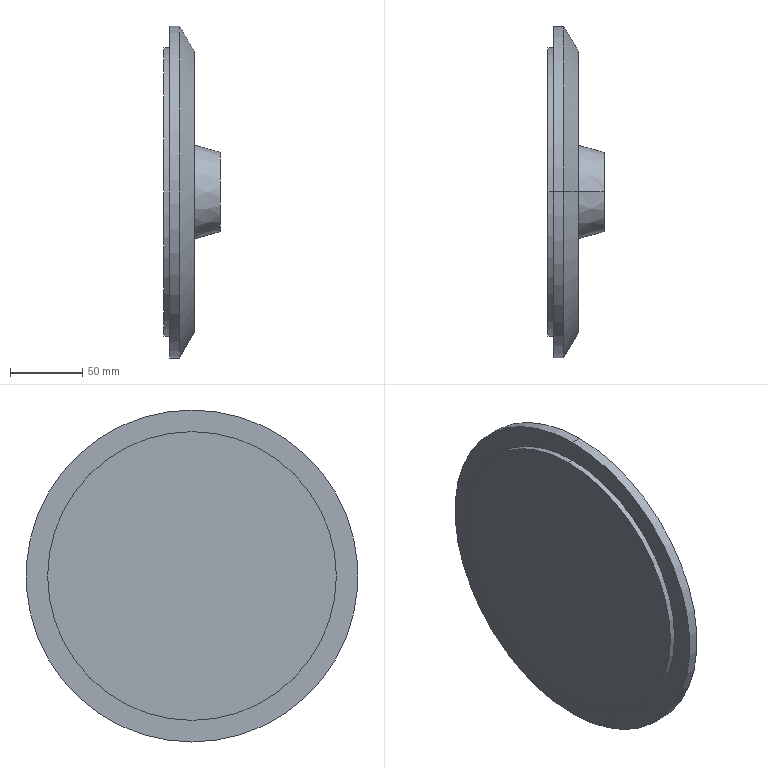Part | SolidWorks | features Revolution 1 | 1 solid | 12 faces | box 39 x 230 x 230 mm | volume 823549 mm3 | cone 4 | cylinder 4 | plane 4 | commonest cylinder face diameters 200 x2 230 x2
STEP:
#1=CARTESIAN_POINT('',(39.,0.,27.5));
#2=VERTEX_POINT('',#1);
#3=CARTESIAN_POINT('',(39.,0.,-27.5));
#4=VERTEX_POINT('',#3);
#5=CARTESIAN_POINT('',(39.,0.,0.));
#6=DIRECTION('',(-1.,0.,0.));
#7=DIRECTION('',(0.,0.,1.));
#8=AXIS2_PLACEMENT_3D('',#5,#6,#7);
#9=CIRCLE('',#8,27.5);
#10=EDGE_CURVE('',#2,#4,#9,.T.);
#11=ORIENTED_EDGE('',*,*,#10,.T.);
#12=CARTESIAN_POINT('',(21.,0.,-32.5));
#13=VERTEX_POINT('',#12);
#14=CARTESIAN_POINT('',(39.,0.,-27.5));
#15=DIRECTION('',(-0.9635,0.,-0.2676));
#16=VECTOR('',#15,1000.);
#17=LINE('',#14,#16);
#18=EDGE_CURVE('',#4,#13,#17,.T.);
#19=ORIENTED_EDGE('',*,*,#18,.T.);
#20=CARTESIAN_POINT('',(21.,0.,32.5));
#21=VERTEX_POINT('',#20);
#22=CARTESIAN_POINT('',(21.,0.,0.));
#23=DIRECTION('',(-1.,0.,0.));
#24=DIRECTION('',(0.,0.,1.));
#25=AXIS2_PLACEMENT_3D('',#22,#23,#24);
#26=CIRCLE('',#25,32.5);
#27=EDGE_CURVE('',#21,#13,#26,.T.);
#28=ORIENTED_EDGE('',*,*,#27,.F.);
#29=CARTESIAN_POINT('',(39.,0.,27.5));
#30=DIRECTION('',(-0.9635,0.,0.2676));
#31=VECTOR('',#30,1000.);
#32=LINE('',#29,#31);
#33=EDGE_CURVE('',#2,#21,#32,.T.);
#34=ORIENTED_EDGE('',*,*,#33,.F.);
#35=EDGE_LOOP('',(#11,#19,#28,#34));
#36=FACE_OUTER_BOUND('',#35,.T.);
#37=CARTESIAN_POINT('',(39.,0.,0.));
#38=DIRECTION('',(-1.,0.,0.));
#39=DIRECTION('',(0.,0.,1.));
#40=AXIS2_PLACEMENT_3D('',#37,#38,#39);
#41=CONICAL_SURFACE('',#40,27.5,0.2709);
#42=ADVANCED_FACE('',(#36),#41,.T.);
#43=CARTESIAN_POINT('',(21.,0.,97.679));
#44=VERTEX_POINT('',#43);
#45=CARTESIAN_POINT('',(21.,0.,-97.679));
#46=VERTEX_POINT('',#45);
#47=CARTESIAN_POINT('',(21.,0.,0.));
#48=DIRECTION('',(-1.,0.,0.));
#49=DIRECTION('',(0.,0.,1.));
#50=AXIS2_PLACEMENT_3D('',#47,#48,#49);
#51=CIRCLE('',#50,97.679);
#52=EDGE_CURVE('',#44,#46,#51,.T.);
#53=ORIENTED_EDGE('',*,*,#52,.T.);
#54=CARTESIAN_POINT('',(11.,0.,-115.));
#55=VERTEX_POINT('',#54);
#56=CARTESIAN_POINT('',(21.,0.,-97.679));
#57=DIRECTION('',(-0.5,0.,-0.866));
#58=VECTOR('',#57,1000.);
#59=LINE('',#56,#58);
#60=EDGE_CURVE('',#46,#55,#59,.T.);
#61=ORIENTED_EDGE('',*,*,#60,.T.);
#62=CARTESIAN_POINT('',(11.,0.,115.));
#63=VERTEX_POINT('',#62);
#64=CARTESIAN_POINT('',(11.,0.,0.));
#65=DIRECTION('',(-1.,0.,0.));
#66=DIRECTION('',(0.,0.,1.));
#67=AXIS2_PLACEMENT_3D('',#64,#65,#66);
#68=CIRCLE('',#67,115.);
#69=EDGE_CURVE('',#63,#55,#68,.T.);
#70=ORIENTED_EDGE('',*,*,#69,.F.);
#71=CARTESIAN_POINT('',(21.,0.,97.679));
#72=DIRECTION('',(-0.5,0.,0.866));
#73=VECTOR('',#72,1000.);
#74=LINE('',#71,#73);
#75=EDGE_CURVE('',#44,#63,#74,.T.);
#76=ORIENTED_EDGE('',*,*,#75,.F.);
#77=EDGE_LOOP('',(#53,#61,#70,#76));
#78=FACE_OUTER_BOUND('',#77,.T.);
#79=CARTESIAN_POINT('',(21.,0.,0.));
#80=DIRECTION('',(-1.,0.,0.));
#81=DIRECTION('',(0.,0.,1.));
#82=AXIS2_PLACEMENT_3D('',#79,#80,#81);
#83=CONICAL_SURFACE('',#82,97.679,1.047);
#84=ADVANCED_FACE('',(#78),#83,.T.);
#85=ORIENTED_EDGE('',*,*,#69,.T.);
#86=CARTESIAN_POINT('',(4.,0.,-115.));
#87=VERTEX_POINT('',#86);
#88=CARTESIAN_POINT('',(0.,0.,-115.));
#89=DIRECTION('',(-1.,0.,0.));
#90=VECTOR('',#89,1000.);
#91=LINE('',#88,#90);
#92=EDGE_CURVE('',#55,#87,#91,.T.);
#93=ORIENTED_EDGE('',*,*,#92,.T.);
#94=CARTESIAN_POINT('',(4.,0.,115.));
#95=VERTEX_POINT('',#94);
#96=CARTESIAN_POINT('',(4.,0.,0.));
#97=DIRECTION('',(-1.,0.,0.));
#98=DIRECTION('',(0.,0.,1.));
#99=AXIS2_PLACEMENT_3D('',#96,#97,#98);
#100=CIRCLE('',#99,115.);
#101=EDGE_CURVE('',#95,#87,#100,.T.);
#102=ORIENTED_EDGE('',*,*,#101,.F.);
#103=CARTESIAN_POINT('',(0.,0.,115.));
#104=DIRECTION('',(-1.,0.,0.));
#105=VECTOR('',#104,1000.);
#106=LINE('',#103,#105);
#107=EDGE_CURVE('',#63,#95,#106,.T.);
#108=ORIENTED_EDGE('',*,*,#107,.F.);
#109=EDGE_LOOP('',(#85,#93,#102,#108));
#110=FACE_OUTER_BOUND('',#109,.T.);
#111=CARTESIAN_POINT('',(0.,0.,0.));
#112=DIRECTION('',(-1.,0.,0.));
#113=DIRECTION('',(0.,0.,1.));
#114=AXIS2_PLACEMENT_3D('',#111,#112,#113);
#115=CYLINDRICAL_SURFACE('',#114,115.);
#116=ADVANCED_FACE('',(#110),#115,.T.);
#117=CARTESIAN_POINT('',(4.,0.,100.));
#118=VERTEX_POINT('',#117);
#119=CARTESIAN_POINT('',(4.,0.,-100.));
#120=VERTEX_POINT('',#119);
#121=CARTESIAN_POINT('',(4.,0.,0.));
#122=DIRECTION('',(-1.,0.,0.));
#123=DIRECTION('',(0.,0.,1.));
#124=AXIS2_PLACEMENT_3D('',#121,#122,#123);
#125=CIRCLE('',#124,100.);
#126=EDGE_CURVE('',#118,#120,#125,.T.);
#127=ORIENTED_EDGE('',*,*,#126,.T.);
#128=CARTESIAN_POINT('',(0.,0.,-100.));
#129=VERTEX_POINT('',#128);
#130=CARTESIAN_POINT('',(0.,0.,-100.));
#131=DIRECTION('',(-1.,0.,0.));
#132=VECTOR('',#131,1000.);
#133=LINE('',#130,#132);
#134=EDGE_CURVE('',#120,#129,#133,.T.);
#135=ORIENTED_EDGE('',*,*,#134,.T.);
#136=CARTESIAN_POINT('',(0.,0.,100.));
#137=VERTEX_POINT('',#136);
#138=CARTESIAN_POINT('',(0.,0.,0.));
#139=DIRECTION('',(-1.,0.,0.));
#140=DIRECTION('',(0.,0.,1.));
#141=AXIS2_PLACEMENT_3D('',#138,#139,#140);
#142=CIRCLE('',#141,100.);
#143=EDGE_CURVE('',#137,#129,#142,.T.);
#144=ORIENTED_EDGE('',*,*,#143,.F.);
#145=CARTESIAN_POINT('',(0.,0.,100.));
#146=DIRECTION('',(-1.,0.,0.));
#147=VECTOR('',#146,1000.);
#148=LINE('',#145,#147);
#149=EDGE_CURVE('',#118,#137,#148,.T.);
#150=ORIENTED_EDGE('',*,*,#149,.F.);
#151=EDGE_LOOP('',(#127,#135,#144,#150));
#152=FACE_OUTER_BOUND('',#151,.T.);
#153=CARTESIAN_POINT('',(0.,0.,0.));
#154=DIRECTION('',(-1.,0.,0.));
#155=DIRECTION('',(0.,0.,1.));
#156=AXIS2_PLACEMENT_3D('',#153,#154,#155);
#157=CYLINDRICAL_SURFACE('',#156,100.);
#158=ADVANCED_FACE('',(#152),#157,.T.);
#159=ORIENTED_EDGE('',*,*,#143,.T.);
#160=CARTESIAN_POINT('',(0.,0.,0.));
#161=DIRECTION('',(-1.,0.,0.));
#162=DIRECTION('',(0.,0.,1.));
#163=AXIS2_PLACEMENT_3D('',#160,#161,#162);
#164=CIRCLE('',#163,100.);
#165=EDGE_CURVE('',#129,#137,#164,.T.);
#166=ORIENTED_EDGE('',*,*,#165,.T.);
#167=EDGE_LOOP('',(#159,#166));
#168=FACE_OUTER_BOUND('',#167,.T.);
#169=CARTESIAN_POINT('',(0.,0.,0.));
#170=DIRECTION('',(1.,0.,0.));
#171=DIRECTION('',(0.,0.,-1.));
#172=AXIS2_PLACEMENT_3D('',#169,#170,#171);
#173=PLANE('',#172);
#174=ADVANCED_FACE('',(#168),#173,.F.);
#175=ORIENTED_EDGE('',*,*,#134,.F.);
#176=CARTESIAN_POINT('',(4.,0.,0.));
#177=DIRECTION('',(-1.,0.,0.));
#178=DIRECTION('',(0.,0.,1.));
#179=AXIS2_PLACEMENT_3D('',#176,#177,#178);
#180=CIRCLE('',#179,100.);
#181=EDGE_CURVE('',#120,#118,#180,.T.);
#182=ORIENTED_EDGE('',*,*,#181,.T.);
#183=ORIENTED_EDGE('',*,*,#149,.T.);
#184=ORIENTED_EDGE('',*,*,#165,.F.);
#185=EDGE_LOOP('',(#175,#182,#183,#184));
#186=FACE_OUTER_BOUND('',#185,.T.);
#187=CARTESIAN_POINT('',(0.,0.,0.));
#188=DIRECTION('',(-1.,0.,0.));
#189=DIRECTION('',(0.,0.,1.));
#190=AXIS2_PLACEMENT_3D('',#187,#188,#189);
#191=CYLINDRICAL_SURFACE('',#190,100.);
#192=ADVANCED_FACE('',(#186),#191,.T.);
#193=ORIENTED_EDGE('',*,*,#126,.F.);
#194=ORIENTED_EDGE('',*,*,#181,.F.);
#195=EDGE_LOOP('',(#193,#194));
#196=FACE_BOUND('',#195,.T.);
#197=ORIENTED_EDGE('',*,*,#101,.T.);
#198=CARTESIAN_POINT('',(4.,0.,0.));
#199=DIRECTION('',(-1.,0.,0.));
#200=DIRECTION('',(0.,0.,1.));
#201=AXIS2_PLACEMENT_3D('',#198,#199,#200);
#202=CIRCLE('',#201,115.);
#203=EDGE_CURVE('',#87,#95,#202,.T.);
#204=ORIENTED_EDGE('',*,*,#203,.T.);
#205=EDGE_LOOP('',(#197,#204));
#206=FACE_OUTER_BOUND('',#205,.T.);
#207=CARTESIAN_POINT('',(4.,100.,0.));
#208=DIRECTION('',(1.,0.,0.));
#209=DIRECTION('',(0.,0.,-1.));
#210=AXIS2_PLACEMENT_3D('',#207,#208,#209);
#211=PLANE('',#210);
#212=ADVANCED_FACE('',(#196,#206),#211,.F.);
#213=ORIENTED_EDGE('',*,*,#92,.F.);
#214=CARTESIAN_POINT('',(11.,0.,0.));
#215=DIRECTION('',(-1.,0.,0.));
#216=DIRECTION('',(0.,0.,1.));
#217=AXIS2_PLACEMENT_3D('',#214,#215,#216);
#218=CIRCLE('',#217,115.);
#219=EDGE_CURVE('',#55,#63,#218,.T.);
#220=ORIENTED_EDGE('',*,*,#219,.T.);
#221=ORIENTED_EDGE('',*,*,#107,.T.);
#222=ORIENTED_EDGE('',*,*,#203,.F.);
#223=EDGE_LOOP('',(#213,#220,#221,#222));
#224=FACE_OUTER_BOUND('',#223,.T.);
#225=CARTESIAN_POINT('',(0.,0.,0.));
#226=DIRECTION('',(-1.,0.,0.));
#227=DIRECTION('',(0.,0.,1.));
#228=AXIS2_PLACEMENT_3D('',#225,#226,#227);
#229=CYLINDRICAL_SURFACE('',#228,115.);
#230=ADVANCED_FACE('',(#224),#229,.T.);
#231=ORIENTED_EDGE('',*,*,#60,.F.);
#232=CARTESIAN_POINT('',(21.,0.,0.));
#233=DIRECTION('',(-1.,0.,0.));
#234=DIRECTION('',(0.,0.,1.));
#235=AXIS2_PLACEMENT_3D('',#232,#233,#234);
#236=CIRCLE('',#235,97.679);
#237=EDGE_CURVE('',#46,#44,#236,.T.);
#238=ORIENTED_EDGE('',*,*,#237,.T.);
#239=ORIENTED_EDGE('',*,*,#75,.T.);
#240=ORIENTED_EDGE('',*,*,#219,.F.);
#241=EDGE_LOOP('',(#231,#238,#239,#240));
#242=FACE_OUTER_BOUND('',#241,.T.);
#243=CARTESIAN_POINT('',(21.,0.,0.));
#244=DIRECTION('',(-1.,0.,0.));
#245=DIRECTION('',(0.,0.,1.));
#246=AXIS2_PLACEMENT_3D('',#243,#244,#245);
#247=CONICAL_SURFACE('',#246,97.679,1.047);
#248=ADVANCED_FACE('',(#242),#247,.T.);
#249=ORIENTED_EDGE('',*,*,#52,.F.);
#250=ORIENTED_EDGE('',*,*,#237,.F.);
#251=EDGE_LOOP('',(#249,#250));
#252=FACE_OUTER_BOUND('',#251,.T.);
#253=ORIENTED_EDGE('',*,*,#27,.T.);
#254=CARTESIAN_POINT('',(21.,0.,0.));
#255=DIRECTION('',(-1.,0.,0.));
#256=DIRECTION('',(0.,0.,1.));
#257=AXIS2_PLACEMENT_3D('',#254,#255,#256);
#258=CIRCLE('',#257,32.5);
#259=EDGE_CURVE('',#13,#21,#258,.T.);
#260=ORIENTED_EDGE('',*,*,#259,.T.);
#261=EDGE_LOOP('',(#253,#260));
#262=FACE_BOUND('',#261,.T.);
#263=CARTESIAN_POINT('',(21.,97.679,0.));
#264=DIRECTION('',(-1.,0.,0.));
#265=DIRECTION('',(0.,0.,1.));
#266=AXIS2_PLACEMENT_3D('',#263,#264,#265);
#267=PLANE('',#266);
#268=ADVANCED_FACE('',(#252,#262),#267,.F.);
#269=ORIENTED_EDGE('',*,*,#18,.F.);
#270=CARTESIAN_POINT('',(39.,0.,0.));
#271=DIRECTION('',(-1.,0.,0.));
#272=DIRECTION('',(0.,0.,1.));
#273=AXIS2_PLACEMENT_3D('',#270,#271,#272);
#274=CIRCLE('',#273,27.5);
#275=EDGE_CURVE('',#4,#2,#274,.T.);
#276=ORIENTED_EDGE('',*,*,#275,.T.);
#277=ORIENTED_EDGE('',*,*,#33,.T.);
#278=ORIENTED_EDGE('',*,*,#259,.F.);
#279=EDGE_LOOP('',(#269,#276,#277,#278));
#280=FACE_OUTER_BOUND('',#279,.T.);
#281=CARTESIAN_POINT('',(39.,0.,0.));
#282=DIRECTION('',(-1.,0.,0.));
#283=DIRECTION('',(0.,0.,1.));
#284=AXIS2_PLACEMENT_3D('',#281,#282,#283);
#285=CONICAL_SURFACE('',#284,27.5,0.2709);
#286=ADVANCED_FACE('',(#280),#285,.T.);
#287=ORIENTED_EDGE('',*,*,#10,.F.);
#288=ORIENTED_EDGE('',*,*,#275,.F.);
#289=EDGE_LOOP('',(#287,#288));
#290=FACE_OUTER_BOUND('',#289,.T.);
#291=CARTESIAN_POINT('',(39.,27.5,0.));
#292=DIRECTION('',(-1.,0.,0.));
#293=DIRECTION('',(0.,0.,1.));
#294=AXIS2_PLACEMENT_3D('',#291,#292,#293);
#295=PLANE('',#294);
#296=ADVANCED_FACE('',(#290),#295,.F.);
#297=CLOSED_SHELL('',(#42,#84,#116,#158,#174,#192,#212,#230,#248,#268,#286,#296));
#298=MANIFOLD_SOLID_BREP('',#297);
#299=CARTESIAN_POINT('',(0.,0.,0.));
#300=DIRECTION('',(0.,0.,1.));
#301=DIRECTION('',(1.,0.,0.));
#302=AXIS2_PLACEMENT_3D('',#299,#300,#301);
#303=(LENGTH_UNIT()NAMED_UNIT(*)SI_UNIT(.MILLI.,.METRE.));
#304=UNCERTAINTY_MEASURE_WITH_UNIT(LENGTH_MEASURE(0.00001),#303,'','');
#305=(NAMED_UNIT(*)PLANE_ANGLE_UNIT()SI_UNIT($,.RADIAN.));
#306=(NAMED_UNIT(*)SI_UNIT($,.STERADIAN.)SOLID_ANGLE_UNIT());
#307=(GEOMETRIC_REPRESENTATION_CONTEXT(3)GLOBAL_UNCERTAINTY_ASSIGNED_CONTEXT((#304))GLOBAL_UNIT_ASSIGNED_CONTEXT((#303,#305,#306))REPRESENTATION_CONTEXT('',''));
#308=ADVANCED_BREP_SHAPE_REPRESENTATION('',(#298,#302),#307);